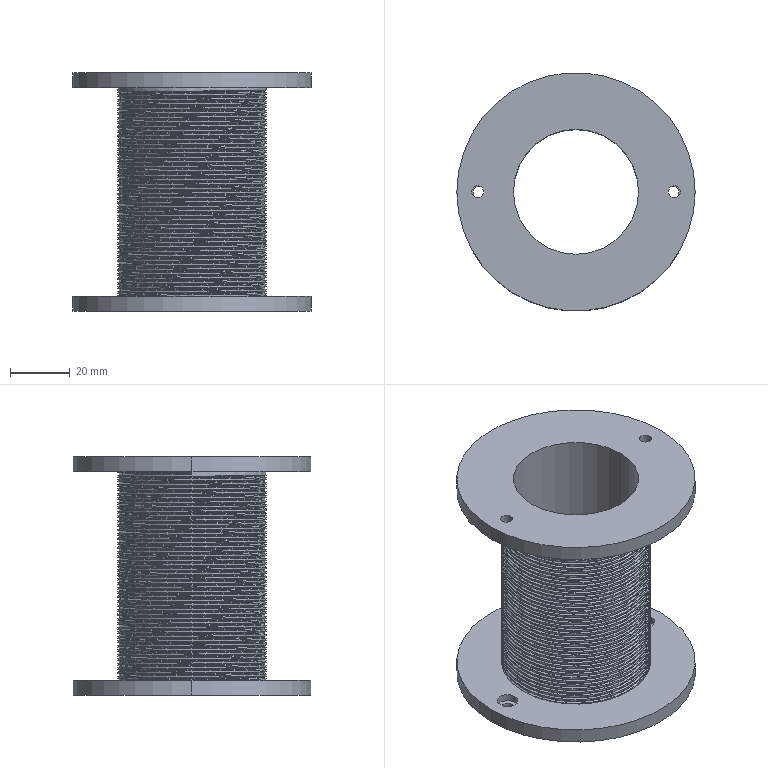Part | STEP file | Load-bearing column 1 | 1 solid | 125 faces | box 80 x 80 x 80 mm | volume 74344 mm3 | cylinder 113 | plane 8 | spline 4 | commonest cylinder face diameters 50 x95 4 x8 7 x4 80 x4 42 x2